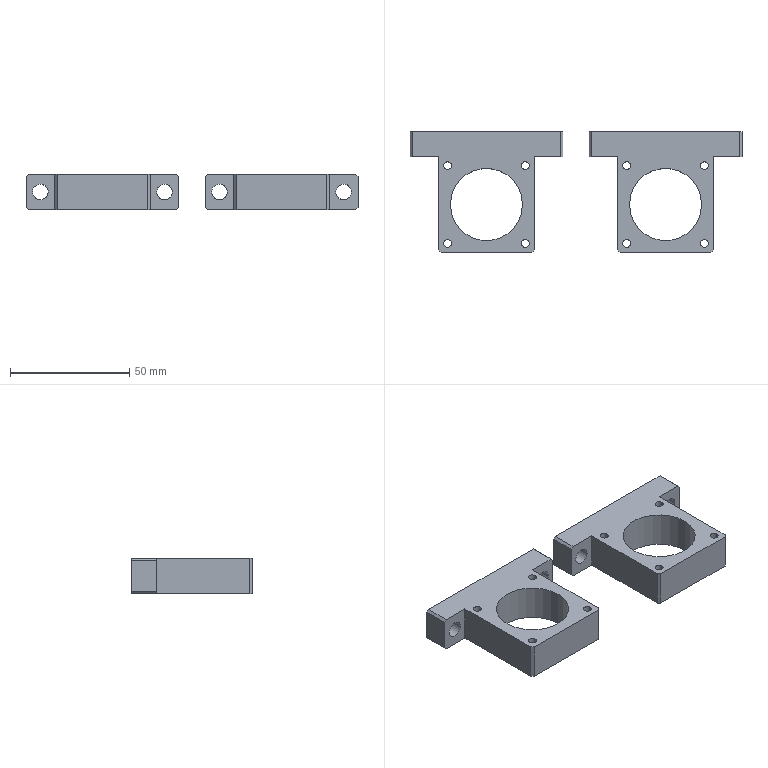CAM job | NX | 3-axis milling, drilling | part box 139 x 50.5 x 15 mm | stock box 144 x 55.5 x 20 mm
Tools:
number,name,description,diameter,corner_radius,flute_length,length,flutes
9,D10,平底铣刀-粗,10.0,0.0,35.0,75.0,2
11,D2-J,平底铣刀-精,2.0,0.0,50.0,75.0,2
7,D6-J,平底铣刀-精,6.0,0.0,25.0,75.0,2
10,D10-J,平底铣刀-精,10.0,0.0,35.0,75.0,2
1,D80R0.8飞刀,圆鼻刀-粗,80.0,0.8,50.0,75.0,2
1,D80R0.8飞刀-J,圆鼻刀-精,80.0,0.8,50.0,75.0,2
2,D6倒角刀,倒角刀,6.0,0.0,3.0,25.0,2
21,M4X0.7,丝锥,3.3,0.0,35.0,50.0,2
13,ZT3.4,钻头,3.4,0.0,35.0,50.0,2
17,ZT10,钻头,10.0,0.0,35.0,50.0,2
Operations:
program,operation,operation_type,tool,method,geometry_group,spindle_rpm,surface_speed,feed_per_tooth,feed_cut,feed_plunge,cut_length_mm,path_length_mm,cut_time_min,machine_time_min
B,底壁铣飞面一刀开粗_COPY,VolumeBased25DMillingOperation,D80R0.8飞刀,分层开粗-切深K-步距G,W-B,2800.0,703.696,0.5357,3000.0,100.0,2224.746,4728.966,0.7416,0.992
B,底壁铣飞面一刀精光_COPY,VolumeBased25DMillingOperation,D80R0.8飞刀-J,侧刃精光-切深K-步距G,W-B,4000.0,1005.28,0.125,1000.0,100.0,246.998,342.998,0.247,0.2566
B,NG_钻倒角_2,Operation,D6倒角刀,METHOD,W-B,8000.0,150.796,0.0625,1000.0,0.0,41.6,442.769,0.0416,0.0817
B,平面去毛刺6X45L_COPY,SurfaceContour,D6倒角刀,爬面_倒角-切深0-步距G,W-B,6500.0,122.519,0.1154,1500.0,100.0,671.255,1462.912,0.4475,0.5267
B,底壁铣倒角_COPY_1,VolumeBased25DMillingOperation,D6倒角刀,爬面_倒角-切深0-步距G,W-B,6500.0,122.519,0.1154,1500.0,100.0,77.202,518.818,0.0515,0.0956
A,顶面,FaceMilling,D80R0.8飞刀,侧刃精光-切深K-步距G,W-A,4500.0,1385.0,0.1667,1500.0,100.0,233.0,329.0,0.1553,0.1649
A,动态开粗D10_COPY,CavityMilling,D10,动态开粗-切深K-步距K,W-A,8000.0,251.32,0.25,4000.0,100.0,6243.724,7034.3,1.561,1.64
A,等高往复层切开粗-中_COPY,ZLevelMilling,D10,分层开粗-切深K-步距G,W-A,8000.0,251.32,0.25,4000.0,100.0,700.631,830.73,0.1752,0.1882
A,打点-深0.8,Operation,D6倒角刀,NONE,W-A,8000.0,150.796,0.0312,500.0,90.0,18.0,409.741,0.036,0.0752
A,通孔-M4螺纹底孔,Operation,ZT3.4,NONE,W-A,3000.0,31.102,0.05,300.0,90.0,176.0,696.739,0.5867,0.6387
A,通孔-精孔12.0预钻,Operation,ZT10,NONE,W-A,800.0,75.398,0.125,200.0,90.0,41.009,258.024,0.205,0.2267
A,铣孔开粗D8_1,CylinderMilling,D10,NONE,W-A,8000.0,251.327,0.125,2000.0,100.0,7108.208,7477.208,3.554,3.591
A,铣孔精光D8-J_1,CylinderMilling,D10-J,精光步距切深关,W-A,8000.0,201.062,0.0312,500.0,100.0,582.468,887.468,1.165,1.195
A,等高光顺清角D2参考6_COPY,ZLevelMilling,D2-J,分层精光-切深K-步距G,W-A,8000.0,50.266,0.125,2000.0,100.0,4051.315,4674.374,2.026,2.088
A,仅选体,SurfaceContour,D6倒角刀,METHOD,W-A,8000.0,150.796,0.1875,3000.0,100.0,634.445,1397.514,0.2115,0.2878
A,NG_钻倒角_1,Operation,D6倒角刀,METHOD,W-A,8000.0,150.796,0.0312,500.0,0.0,41.6,442.769,0.0832,0.1233
A,铣倒角_1,PlanarMilling,D6倒角刀,METHOD,W-A,8000.0,150.796,0.0312,500.0,100.0,201.805,479.045,0.4036,0.4313
A,底壁铣倒角_COPY,VolumeBased25DMillingOperation,D6倒角刀,爬面_倒角-切深0-步距G,W-A,6500.0,122.519,0.1154,1500.0,100.0,77.202,518.818,0.0515,0.0956
A,通孔-攻牙M4,Operation,M4X0.7,METHOD,W-A,600.0,6.22,0.0006,0.7,90.0,152.0,648.739,217.143,217.192
A,外形半精_2,VolumeBased25DMillingOperation,D6-J,METHOD,W-A,9000.0,169.646,0.0667,1200.0,100.0,996.076,1564.634,0.8301,0.8869